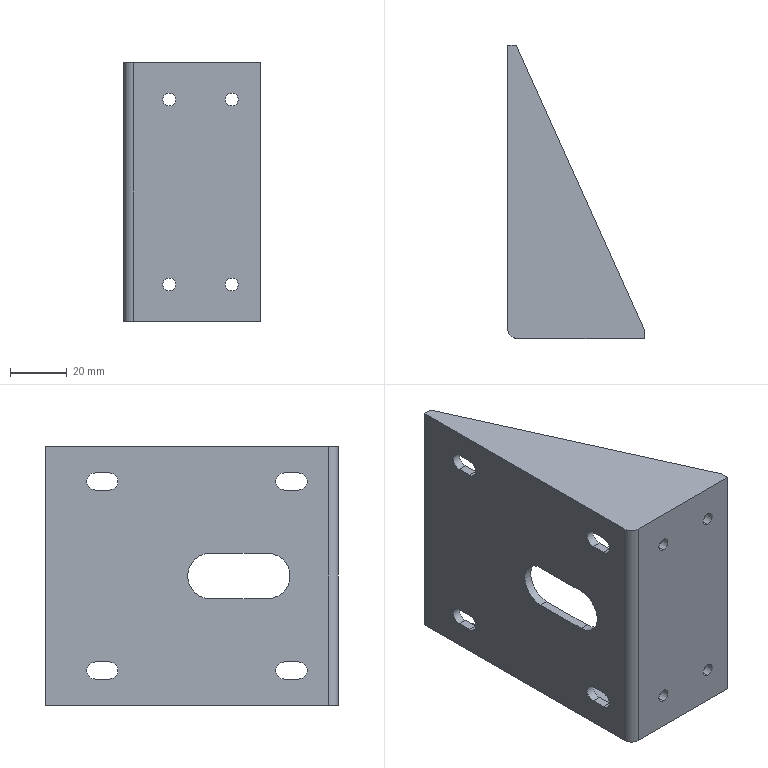Part | SolidWorks | features ICE 4, Cut 1, FlatPattern 1, SMBaseFlange 1, SheetMetal 1 | 1 solid | 42 faces | box 48 x 103 x 91 mm | volume 51216 mm3 | plane 22 | cylinder 20 | commonest cylinder face diameters 4.5 x8 6 x8 16 x2 1 x1 7 x1
STEP:
#1=CARTESIAN_POINT('',(13.,0.,7.75));
#2=VERTEX_POINT('',#1);
#3=CARTESIAN_POINT('',(13.,0.,12.25));
#4=VERTEX_POINT('',#3);
#5=CARTESIAN_POINT('',(13.,0.,10.));
#6=DIRECTION('',(0.,1.,0.));
#7=DIRECTION('',(0.,0.,1.));
#8=AXIS2_PLACEMENT_3D('',#5,#6,#7);
#9=CIRCLE('',#8,2.25);
#10=EDGE_CURVE('',#2,#4,#9,.T.);
#11=ORIENTED_EDGE('',*,*,#10,.T.);
#12=CARTESIAN_POINT('',(13.,-3.,12.25));
#13=VERTEX_POINT('',#12);
#14=CARTESIAN_POINT('',(13.,100.,12.25));
#15=DIRECTION('',(0.,-1.,0.));
#16=VECTOR('',#15,1000.);
#17=LINE('',#14,#16);
#18=EDGE_CURVE('',#4,#13,#17,.T.);
#19=ORIENTED_EDGE('',*,*,#18,.T.);
#20=CARTESIAN_POINT('',(13.,-3.,7.75));
#21=VERTEX_POINT('',#20);
#22=CARTESIAN_POINT('',(13.,-3.,10.));
#23=DIRECTION('',(0.,-1.,0.));
#24=DIRECTION('',(0.,0.,-1.));
#25=AXIS2_PLACEMENT_3D('',#22,#23,#24);
#26=CIRCLE('',#25,2.25);
#27=EDGE_CURVE('',#13,#21,#26,.T.);
#28=ORIENTED_EDGE('',*,*,#27,.T.);
#29=CARTESIAN_POINT('',(13.,100.,7.75));
#30=DIRECTION('',(0.,-1.,0.));
#31=VECTOR('',#30,1000.);
#32=LINE('',#29,#31);
#33=EDGE_CURVE('',#2,#21,#32,.T.);
#34=ORIENTED_EDGE('',*,*,#33,.F.);
#35=EDGE_LOOP('',(#11,#19,#28,#34));
#36=FACE_OUTER_BOUND('',#35,.T.);
#37=CARTESIAN_POINT('',(13.,100.,10.));
#38=DIRECTION('',(0.,-1.,0.));
#39=DIRECTION('',(0.,0.,-1.));
#40=AXIS2_PLACEMENT_3D('',#37,#38,#39);
#41=CYLINDRICAL_SURFACE('',#40,2.25);
#42=ADVANCED_FACE('',(#36),#41,.F.);
#43=CARTESIAN_POINT('',(35.,0.,7.75));
#44=VERTEX_POINT('',#43);
#45=CARTESIAN_POINT('',(35.,0.,12.25));
#46=VERTEX_POINT('',#45);
#47=CARTESIAN_POINT('',(35.,0.,10.));
#48=DIRECTION('',(0.,1.,0.));
#49=DIRECTION('',(0.,0.,1.));
#50=AXIS2_PLACEMENT_3D('',#47,#48,#49);
#51=CIRCLE('',#50,2.25);
#52=EDGE_CURVE('',#44,#46,#51,.T.);
#53=ORIENTED_EDGE('',*,*,#52,.T.);
#54=CARTESIAN_POINT('',(35.,-3.,12.25));
#55=VERTEX_POINT('',#54);
#56=CARTESIAN_POINT('',(35.,100.,12.25));
#57=DIRECTION('',(0.,-1.,0.));
#58=VECTOR('',#57,1000.);
#59=LINE('',#56,#58);
#60=EDGE_CURVE('',#46,#55,#59,.T.);
#61=ORIENTED_EDGE('',*,*,#60,.T.);
#62=CARTESIAN_POINT('',(35.,-3.,7.75));
#63=VERTEX_POINT('',#62);
#64=CARTESIAN_POINT('',(35.,-3.,10.));
#65=DIRECTION('',(0.,-1.,0.));
#66=DIRECTION('',(0.,0.,-1.));
#67=AXIS2_PLACEMENT_3D('',#64,#65,#66);
#68=CIRCLE('',#67,2.25);
#69=EDGE_CURVE('',#55,#63,#68,.T.);
#70=ORIENTED_EDGE('',*,*,#69,.T.);
#71=CARTESIAN_POINT('',(35.,100.,7.75));
#72=DIRECTION('',(0.,-1.,0.));
#73=VECTOR('',#72,1000.);
#74=LINE('',#71,#73);
#75=EDGE_CURVE('',#44,#63,#74,.T.);
#76=ORIENTED_EDGE('',*,*,#75,.F.);
#77=EDGE_LOOP('',(#53,#61,#70,#76));
#78=FACE_OUTER_BOUND('',#77,.T.);
#79=CARTESIAN_POINT('',(35.,100.,10.));
#80=DIRECTION('',(0.,-1.,0.));
#81=DIRECTION('',(0.,0.,-1.));
#82=AXIS2_PLACEMENT_3D('',#79,#80,#81);
#83=CYLINDRICAL_SURFACE('',#82,2.25);
#84=ADVANCED_FACE('',(#78),#83,.F.);
#85=CARTESIAN_POINT('',(35.,0.,72.75));
#86=VERTEX_POINT('',#85);
#87=CARTESIAN_POINT('',(35.,0.,77.25));
#88=VERTEX_POINT('',#87);
#89=CARTESIAN_POINT('',(35.,0.,75.));
#90=DIRECTION('',(0.,1.,0.));
#91=DIRECTION('',(0.,0.,1.));
#92=AXIS2_PLACEMENT_3D('',#89,#90,#91);
#93=CIRCLE('',#92,2.25);
#94=EDGE_CURVE('',#86,#88,#93,.T.);
#95=ORIENTED_EDGE('',*,*,#94,.T.);
#96=CARTESIAN_POINT('',(35.,-3.,77.25));
#97=VERTEX_POINT('',#96);
#98=CARTESIAN_POINT('',(35.,100.,77.25));
#99=DIRECTION('',(0.,-1.,0.));
#100=VECTOR('',#99,1000.);
#101=LINE('',#98,#100);
#102=EDGE_CURVE('',#88,#97,#101,.T.);
#103=ORIENTED_EDGE('',*,*,#102,.T.);
#104=CARTESIAN_POINT('',(35.,-3.,72.75));
#105=VERTEX_POINT('',#104);
#106=CARTESIAN_POINT('',(35.,-3.,75.));
#107=DIRECTION('',(0.,-1.,0.));
#108=DIRECTION('',(0.,0.,-1.));
#109=AXIS2_PLACEMENT_3D('',#106,#107,#108);
#110=CIRCLE('',#109,2.25);
#111=EDGE_CURVE('',#97,#105,#110,.T.);
#112=ORIENTED_EDGE('',*,*,#111,.T.);
#113=CARTESIAN_POINT('',(35.,100.,72.75));
#114=DIRECTION('',(0.,-1.,0.));
#115=VECTOR('',#114,1000.);
#116=LINE('',#113,#115);
#117=EDGE_CURVE('',#86,#105,#116,.T.);
#118=ORIENTED_EDGE('',*,*,#117,.F.);
#119=EDGE_LOOP('',(#95,#103,#112,#118));
#120=FACE_OUTER_BOUND('',#119,.T.);
#121=CARTESIAN_POINT('',(35.,100.,75.));
#122=DIRECTION('',(0.,-1.,0.));
#123=DIRECTION('',(0.,0.,-1.));
#124=AXIS2_PLACEMENT_3D('',#121,#122,#123);
#125=CYLINDRICAL_SURFACE('',#124,2.25);
#126=ADVANCED_FACE('',(#120),#125,.F.);
#127=CARTESIAN_POINT('',(13.,0.,72.75));
#128=VERTEX_POINT('',#127);
#129=CARTESIAN_POINT('',(13.,0.,77.25));
#130=VERTEX_POINT('',#129);
#131=CARTESIAN_POINT('',(13.,0.,75.));
#132=DIRECTION('',(0.,1.,0.));
#133=DIRECTION('',(0.,0.,1.));
#134=AXIS2_PLACEMENT_3D('',#131,#132,#133);
#135=CIRCLE('',#134,2.25);
#136=EDGE_CURVE('',#128,#130,#135,.T.);
#137=ORIENTED_EDGE('',*,*,#136,.T.);
#138=CARTESIAN_POINT('',(13.,-3.,77.25));
#139=VERTEX_POINT('',#138);
#140=CARTESIAN_POINT('',(13.,100.,77.25));
#141=DIRECTION('',(0.,-1.,0.));
#142=VECTOR('',#141,1000.);
#143=LINE('',#140,#142);
#144=EDGE_CURVE('',#130,#139,#143,.T.);
#145=ORIENTED_EDGE('',*,*,#144,.T.);
#146=CARTESIAN_POINT('',(13.,-3.,72.75));
#147=VERTEX_POINT('',#146);
#148=CARTESIAN_POINT('',(13.,-3.,75.));
#149=DIRECTION('',(0.,-1.,0.));
#150=DIRECTION('',(0.,0.,-1.));
#151=AXIS2_PLACEMENT_3D('',#148,#149,#150);
#152=CIRCLE('',#151,2.25);
#153=EDGE_CURVE('',#139,#147,#152,.T.);
#154=ORIENTED_EDGE('',*,*,#153,.T.);
#155=CARTESIAN_POINT('',(13.,100.,72.75));
#156=DIRECTION('',(0.,-1.,0.));
#157=VECTOR('',#156,1000.);
#158=LINE('',#155,#157);
#159=EDGE_CURVE('',#128,#147,#158,.T.);
#160=ORIENTED_EDGE('',*,*,#159,.F.);
#161=EDGE_LOOP('',(#137,#145,#154,#160));
#162=FACE_OUTER_BOUND('',#161,.T.);
#163=CARTESIAN_POINT('',(13.,100.,75.));
#164=DIRECTION('',(0.,-1.,0.));
#165=DIRECTION('',(0.,0.,-1.));
#166=AXIS2_PLACEMENT_3D('',#163,#164,#165);
#167=CYLINDRICAL_SURFACE('',#166,2.25);
#168=ADVANCED_FACE('',(#162),#167,.F.);
#169=CARTESIAN_POINT('',(13.,-3.,10.));
#170=DIRECTION('',(0.,-1.,0.));
#171=DIRECTION('',(0.,0.,-1.));
#172=AXIS2_PLACEMENT_3D('',#169,#170,#171);
#173=CIRCLE('',#172,2.25);
#174=EDGE_CURVE('',#21,#13,#173,.T.);
#175=ORIENTED_EDGE('',*,*,#174,.F.);
#176=ORIENTED_EDGE('',*,*,#27,.F.);
#177=EDGE_LOOP('',(#175,#176));
#178=FACE_BOUND('',#177,.T.);
#179=CARTESIAN_POINT('',(35.,-3.,10.));
#180=DIRECTION('',(0.,-1.,0.));
#181=DIRECTION('',(0.,0.,-1.));
#182=AXIS2_PLACEMENT_3D('',#179,#180,#181);
#183=CIRCLE('',#182,2.25);
#184=EDGE_CURVE('',#63,#55,#183,.T.);
#185=ORIENTED_EDGE('',*,*,#184,.F.);
#186=ORIENTED_EDGE('',*,*,#69,.F.);
#187=EDGE_LOOP('',(#185,#186));
#188=FACE_BOUND('',#187,.T.);
#189=CARTESIAN_POINT('',(35.,-3.,75.));
#190=DIRECTION('',(0.,-1.,0.));
#191=DIRECTION('',(0.,0.,-1.));
#192=AXIS2_PLACEMENT_3D('',#189,#190,#191);
#193=CIRCLE('',#192,2.25);
#194=EDGE_CURVE('',#105,#97,#193,.T.);
#195=ORIENTED_EDGE('',*,*,#194,.F.);
#196=ORIENTED_EDGE('',*,*,#111,.F.);
#197=EDGE_LOOP('',(#195,#196));
#198=FACE_BOUND('',#197,.T.);
#199=CARTESIAN_POINT('',(13.,-3.,75.));
#200=DIRECTION('',(0.,-1.,0.));
#201=DIRECTION('',(0.,0.,-1.));
#202=AXIS2_PLACEMENT_3D('',#199,#200,#201);
#203=CIRCLE('',#202,2.25);
#204=EDGE_CURVE('',#147,#139,#203,.T.);
#205=ORIENTED_EDGE('',*,*,#204,.F.);
#206=ORIENTED_EDGE('',*,*,#153,.F.);
#207=EDGE_LOOP('',(#205,#206));
#208=FACE_BOUND('',#207,.T.);
#209=CARTESIAN_POINT('',(0.5,-3.,88.));
#210=VERTEX_POINT('',#209);
#211=CARTESIAN_POINT('',(0.5,-3.,-3.));
#212=VERTEX_POINT('',#211);
#213=CARTESIAN_POINT('',(0.5,-3.,85.));
#214=DIRECTION('',(0.,0.,-1.));
#215=VECTOR('',#214,1000.);
#216=LINE('',#213,#215);
#217=EDGE_CURVE('',#210,#212,#216,.T.);
#218=ORIENTED_EDGE('',*,*,#217,.T.);
#219=CARTESIAN_POINT('',(45.,-3.,-3.));
#220=VERTEX_POINT('',#219);
#221=CARTESIAN_POINT('',(45.,-3.,-3.));
#222=DIRECTION('',(-1.,0.,0.));
#223=VECTOR('',#222,1000.);
#224=LINE('',#221,#223);
#225=EDGE_CURVE('',#220,#212,#224,.T.);
#226=ORIENTED_EDGE('',*,*,#225,.F.);
#227=CARTESIAN_POINT('',(45.,-3.,88.));
#228=VERTEX_POINT('',#227);
#229=CARTESIAN_POINT('',(45.,-3.,85.));
#230=DIRECTION('',(0.,0.,-1.));
#231=VECTOR('',#230,1000.);
#232=LINE('',#229,#231);
#233=EDGE_CURVE('',#228,#220,#232,.T.);
#234=ORIENTED_EDGE('',*,*,#233,.F.);
#235=CARTESIAN_POINT('',(45.,-3.,88.));
#236=DIRECTION('',(1.,0.,0.));
#237=VECTOR('',#236,1000.);
#238=LINE('',#235,#237);
#239=EDGE_CURVE('',#210,#228,#238,.T.);
#240=ORIENTED_EDGE('',*,*,#239,.F.);
#241=EDGE_LOOP('',(#218,#226,#234,#240));
#242=FACE_OUTER_BOUND('',#241,.T.);
#243=CARTESIAN_POINT('',(0.,-3.,85.));
#244=DIRECTION('',(0.,1.,0.));
#245=DIRECTION('',(0.,0.,1.));
#246=AXIS2_PLACEMENT_3D('',#243,#244,#245);
#247=PLANE('',#246);
#248=ADVANCED_FACE('',(#178,#188,#198,#208,#242),#247,.F.);
#249=ORIENTED_EDGE('',*,*,#233,.T.);
#250=CARTESIAN_POINT('',(45.,0.,-3.));
#251=VERTEX_POINT('',#250);
#252=CARTESIAN_POINT('',(45.,0.,-3.));
#253=DIRECTION('',(0.,-1.,0.));
#254=VECTOR('',#253,1000.);
#255=LINE('',#252,#254);
#256=EDGE_CURVE('',#251,#220,#255,.T.);
#257=ORIENTED_EDGE('',*,*,#256,.F.);
#258=CARTESIAN_POINT('',(45.,0.,0.));
#259=VERTEX_POINT('',#258);
#260=CARTESIAN_POINT('',(45.,0.,-3.));
#261=DIRECTION('',(0.,0.,1.));
#262=VECTOR('',#261,1000.);
#263=LINE('',#260,#262);
#264=EDGE_CURVE('',#251,#259,#263,.T.);
#265=ORIENTED_EDGE('',*,*,#264,.T.);
#266=CARTESIAN_POINT('',(45.,0.,85.));
#267=VERTEX_POINT('',#266);
#268=CARTESIAN_POINT('',(45.,0.,85.));
#269=DIRECTION('',(0.,0.,-1.));
#270=VECTOR('',#269,1000.);
#271=LINE('',#268,#270);
#272=EDGE_CURVE('',#267,#259,#271,.T.);
#273=ORIENTED_EDGE('',*,*,#272,.F.);
#274=CARTESIAN_POINT('',(45.,0.,88.));
#275=VERTEX_POINT('',#274);
#276=CARTESIAN_POINT('',(45.,0.,88.));
#277=DIRECTION('',(0.,0.,-1.));
#278=VECTOR('',#277,1000.);
#279=LINE('',#276,#278);
#280=EDGE_CURVE('',#275,#267,#279,.T.);
#281=ORIENTED_EDGE('',*,*,#280,.F.);
#282=CARTESIAN_POINT('',(45.,0.,88.));
#283=DIRECTION('',(0.,1.,0.));
#284=VECTOR('',#283,1000.);
#285=LINE('',#282,#284);
#286=EDGE_CURVE('',#228,#275,#285,.T.);
#287=ORIENTED_EDGE('',*,*,#286,.F.);
#288=EDGE_LOOP('',(#249,#257,#265,#273,#281,#287));
#289=FACE_OUTER_BOUND('',#288,.T.);
#290=CARTESIAN_POINT('',(45.,0.,85.));
#291=DIRECTION('',(1.,0.,0.));
#292=DIRECTION('',(0.,0.,-1.));
#293=AXIS2_PLACEMENT_3D('',#290,#291,#292);
#294=PLANE('',#293);
#295=ADVANCED_FACE('',(#289),#294,.T.);
#296=ORIENTED_EDGE('',*,*,#10,.F.);
#297=CARTESIAN_POINT('',(13.,0.,10.));
#298=DIRECTION('',(0.,1.,0.));
#299=DIRECTION('',(0.,0.,1.));
#300=AXIS2_PLACEMENT_3D('',#297,#298,#299);
#301=CIRCLE('',#300,2.25);
#302=EDGE_CURVE('',#4,#2,#301,.T.);
#303=ORIENTED_EDGE('',*,*,#302,.F.);
#304=EDGE_LOOP('',(#296,#303));
#305=FACE_BOUND('',#304,.T.);
#306=ORIENTED_EDGE('',*,*,#52,.F.);
#307=CARTESIAN_POINT('',(35.,0.,10.));
#308=DIRECTION('',(0.,1.,0.));
#309=DIRECTION('',(0.,0.,1.));
#310=AXIS2_PLACEMENT_3D('',#307,#308,#309);
#311=CIRCLE('',#310,2.25);
#312=EDGE_CURVE('',#46,#44,#311,.T.);
#313=ORIENTED_EDGE('',*,*,#312,.F.);
#314=EDGE_LOOP('',(#306,#313));
#315=FACE_BOUND('',#314,.T.);
#316=ORIENTED_EDGE('',*,*,#94,.F.);
#317=CARTESIAN_POINT('',(35.,0.,75.));
#318=DIRECTION('',(0.,1.,0.));
#319=DIRECTION('',(0.,0.,1.));
#320=AXIS2_PLACEMENT_3D('',#317,#318,#319);
#321=CIRCLE('',#320,2.25);
#322=EDGE_CURVE('',#88,#86,#321,.T.);
#323=ORIENTED_EDGE('',*,*,#322,.F.);
#324=EDGE_LOOP('',(#316,#323));
#325=FACE_BOUND('',#324,.T.);
#326=ORIENTED_EDGE('',*,*,#136,.F.);
#327=CARTESIAN_POINT('',(13.,0.,75.));
#328=DIRECTION('',(0.,1.,0.));
#329=DIRECTION('',(0.,0.,1.));
#330=AXIS2_PLACEMENT_3D('',#327,#328,#329);
#331=CIRCLE('',#330,2.25);
#332=EDGE_CURVE('',#130,#128,#331,.T.);
#333=ORIENTED_EDGE('',*,*,#332,.F.);
#334=EDGE_LOOP('',(#326,#333));
#335=FACE_BOUND('',#334,.T.);
#336=CARTESIAN_POINT('',(0.5,0.,0.));
#337=VERTEX_POINT('',#336);
#338=CARTESIAN_POINT('',(0.,0.,0.));
#339=DIRECTION('',(1.,0.,0.));
#340=VECTOR('',#339,1000.);
#341=LINE('',#338,#340);
#342=EDGE_CURVE('',#337,#259,#341,.T.);
#343=ORIENTED_EDGE('',*,*,#342,.F.);
#344=CARTESIAN_POINT('',(0.5,0.,85.));
#345=VERTEX_POINT('',#344);
#346=CARTESIAN_POINT('',(0.5,0.,85.));
#347=DIRECTION('',(0.,0.,-1.));
#348=VECTOR('',#347,1000.);
#349=LINE('',#346,#348);
#350=EDGE_CURVE('',#345,#337,#349,.T.);
#351=ORIENTED_EDGE('',*,*,#350,.F.);
#352=CARTESIAN_POINT('',(0.,0.,85.));
#353=DIRECTION('',(1.,0.,0.));
#354=VECTOR('',#353,1000.);
#355=LINE('',#352,#354);
#356=EDGE_CURVE('',#345,#267,#355,.T.);
#357=ORIENTED_EDGE('',*,*,#356,.T.);
#358=ORIENTED_EDGE('',*,*,#272,.T.);
#359=EDGE_LOOP('',(#343,#351,#357,#358));
#360=FACE_OUTER_BOUND('',#359,.T.);
#361=CARTESIAN_POINT('',(0.,0.,85.));
#362=DIRECTION('',(0.,1.,0.));
#363=DIRECTION('',(0.,0.,1.));
#364=AXIS2_PLACEMENT_3D('',#361,#362,#363);
#365=PLANE('',#364);
#366=ADVANCED_FACE('',(#305,#315,#325,#335,#360),#365,.T.);
#367=CARTESIAN_POINT('',(0.,0.5,0.));
#368=VERTEX_POINT('',#367);
#369=CARTESIAN_POINT('',(0.5,0.5,0.));
#370=DIRECTION('',(0.,0.,1.));
#371=DIRECTION('',(-1.,0.,0.));
#372=AXIS2_PLACEMENT_3D('',#369,#370,#371);
#373=CIRCLE('',#372,0.5);
#374=EDGE_CURVE('',#368,#337,#373,.T.);
#375=ORIENTED_EDGE('',*,*,#374,.F.);
#376=CARTESIAN_POINT('',(0.,0.5,85.));
#377=VERTEX_POINT('',#376);
#378=CARTESIAN_POINT('',(0.,0.5,85.));
#379=DIRECTION('',(0.,0.,-1.));
#380=VECTOR('',#379,1000.);
#381=LINE('',#378,#380);
#382=EDGE_CURVE('',#377,#368,#381,.T.);
#383=ORIENTED_EDGE('',*,*,#382,.F.);
#384=CARTESIAN_POINT('',(0.5,0.5,85.));
#385=DIRECTION('',(0.,0.,1.));
#386=DIRECTION('',(-1.,0.,0.));
#387=AXIS2_PLACEMENT_3D('',#384,#385,#386);
#388=CIRCLE('',#387,0.5);
#389=EDGE_CURVE('',#377,#345,#388,.T.);
#390=ORIENTED_EDGE('',*,*,#389,.T.);
#391=ORIENTED_EDGE('',*,*,#350,.T.);
#392=EDGE_LOOP('',(#375,#383,#390,#391));
#393=FACE_OUTER_BOUND('',#392,.T.);
#394=CARTESIAN_POINT('',(0.5,0.5,85.));
#395=DIRECTION('',(0.,0.,-1.));
#396=DIRECTION('',(-1.,0.,0.));
#397=AXIS2_PLACEMENT_3D('',#394,#395,#396);
#398=CYLINDRICAL_SURFACE('',#397,0.5);
#399=ADVANCED_FACE('',(#393),#398,.F.);
#400=CARTESIAN_POINT('',(0.,22.,50.5));
#401=VERTEX_POINT('',#400);
#402=CARTESIAN_POINT('',(0.,22.,34.5));
#403=VERTEX_POINT('',#402);
#404=CARTESIAN_POINT('',(0.,22.,42.5));
#405=DIRECTION('',(1.,0.,0.));
#406=DIRECTION('',(0.,0.,-1.));
#407=AXIS2_PLACEMENT_3D('',#404,#405,#406);
#408=CIRCLE('',#407,8.);
#409=EDGE_CURVE('',#401,#403,#408,.T.);
#410=ORIENTED_EDGE('',*,*,#409,.F.);
#411=CARTESIAN_POINT('',(0.,42.,50.5));
#412=VERTEX_POINT('',#411);
#413=CARTESIAN_POINT('',(0.,0.,50.5));
#414=DIRECTION('',(0.,-1.,0.));
#415=VECTOR('',#414,1000.);
#416=LINE('',#413,#415);
#417=EDGE_CURVE('',#412,#401,#416,.T.);
#418=ORIENTED_EDGE('',*,*,#417,.F.);
#419=CARTESIAN_POINT('',(0.,42.,34.5));
#420=VERTEX_POINT('',#419);
#421=CARTESIAN_POINT('',(0.,42.,42.5));
#422=DIRECTION('',(1.,0.,0.));
#423=DIRECTION('',(0.,0.,-1.));
#424=AXIS2_PLACEMENT_3D('',#421,#422,#423);
#425=CIRCLE('',#424,8.);
#426=EDGE_CURVE('',#420,#412,#425,.T.);
#427=ORIENTED_EDGE('',*,*,#426,.F.);
#428=CARTESIAN_POINT('',(0.,0.,34.5));
#429=DIRECTION('',(0.,1.,0.));
#430=VECTOR('',#429,1000.);
#431=LINE('',#428,#430);
#432=EDGE_CURVE('',#403,#420,#431,.T.);
#433=ORIENTED_EDGE('',*,*,#432,.F.);
#434=EDGE_LOOP('',(#410,#418,#427,#433));
#435=FACE_BOUND('',#434,.T.);
#436=CARTESIAN_POINT('',(0.,16.03,6.265));
#437=VERTEX_POINT('',#436);
#438=CARTESIAN_POINT('',(0.,16.03,12.265));
#439=VERTEX_POINT('',#438);
#440=CARTESIAN_POINT('',(0.,16.03,9.265));
#441=DIRECTION('',(1.,0.,0.));
#442=DIRECTION('',(0.,0.,-1.));
#443=AXIS2_PLACEMENT_3D('',#440,#441,#442);
#444=CIRCLE('',#443,3.);
#445=EDGE_CURVE('',#437,#439,#444,.T.);
#446=ORIENTED_EDGE('',*,*,#445,.F.);
#447=CARTESIAN_POINT('',(0.,11.03,6.265));
#448=VERTEX_POINT('',#447);
#449=CARTESIAN_POINT('',(0.,0.,6.265));
#450=DIRECTION('',(0.,1.,0.));
#451=VECTOR('',#450,1000.);
#452=LINE('',#449,#451);
#453=EDGE_CURVE('',#448,#437,#452,.T.);
#454=ORIENTED_EDGE('',*,*,#453,.F.);
#455=CARTESIAN_POINT('',(0.,11.03,12.265));
#456=VERTEX_POINT('',#455);
#457=CARTESIAN_POINT('',(0.,11.03,9.265));
#458=DIRECTION('',(1.,0.,0.));
#459=DIRECTION('',(0.,0.,-1.));
#460=AXIS2_PLACEMENT_3D('',#457,#458,#459);
#461=CIRCLE('',#460,3.);
#462=EDGE_CURVE('',#456,#448,#461,.T.);
#463=ORIENTED_EDGE('',*,*,#462,.F.);
#464=CARTESIAN_POINT('',(0.,0.,12.265));
#465=DIRECTION('',(0.,-1.,0.));
#466=VECTOR('',#465,1000.);
#467=LINE('',#464,#466);
#468=EDGE_CURVE('',#439,#456,#467,.T.);
#469=ORIENTED_EDGE('',*,*,#468,.F.);
#470=EDGE_LOOP('',(#446,#454,#463,#469));
#471=FACE_BOUND('',#470,.T.);
#472=CARTESIAN_POINT('',(0.,16.03,72.735));
#473=VERTEX_POINT('',#472);
#474=CARTESIAN_POINT('',(0.,16.03,78.735));
#475=VERTEX_POINT('',#474);
#476=CARTESIAN_POINT('',(0.,16.03,75.735));
#477=DIRECTION('',(1.,0.,0.));
#478=DIRECTION('',(0.,0.,-1.));
#479=AXIS2_PLACEMENT_3D('',#476,#477,#478);
#480=CIRCLE('',#479,3.);
#481=EDGE_CURVE('',#473,#475,#480,.T.);
#482=ORIENTED_EDGE('',*,*,#481,.F.);
#483=CARTESIAN_POINT('',(0.,11.03,72.735));
#484=VERTEX_POINT('',#483);
#485=CARTESIAN_POINT('',(0.,0.,72.735));
#486=DIRECTION('',(0.,1.,0.));
#487=VECTOR('',#486,1000.);
#488=LINE('',#485,#487);
#489=EDGE_CURVE('',#484,#473,#488,.T.);
#490=ORIENTED_EDGE('',*,*,#489,.F.);
#491=CARTESIAN_POINT('',(0.,11.03,78.735));
#492=VERTEX_POINT('',#491);
#493=CARTESIAN_POINT('',(0.,11.03,75.735));
#494=DIRECTION('',(1.,0.,0.));
#495=DIRECTION('',(0.,0.,-1.));
#496=AXIS2_PLACEMENT_3D('',#493,#494,#495);
#497=CIRCLE('',#496,3.);
#498=EDGE_CURVE('',#492,#484,#497,.T.);
#499=ORIENTED_EDGE('',*,*,#498,.F.);
#500=CARTESIAN_POINT('',(0.,0.,78.735));
#501=DIRECTION('',(0.,-1.,0.));
#502=VECTOR('',#501,1000.);
#503=LINE('',#500,#502);
#504=EDGE_CURVE('',#475,#492,#503,.T.);
#505=ORIENTED_EDGE('',*,*,#504,.F.);
#506=EDGE_LOOP('',(#482,#490,#499,#505));
#507=FACE_BOUND('',#506,.T.);
#508=CARTESIAN_POINT('',(0.,82.5,72.735));
#509=VERTEX_POINT('',#508);
#510=CARTESIAN_POINT('',(0.,82.5,78.735));
#511=VERTEX_POINT('',#510);
#512=CARTESIAN_POINT('',(0.,82.5,75.735));
#513=DIRECTION('',(1.,0.,0.));
#514=DIRECTION('',(0.,0.,-1.));
#515=AXIS2_PLACEMENT_3D('',#512,#513,#514);
#516=CIRCLE('',#515,3.);
#517=EDGE_CURVE('',#509,#511,#516,.T.);
#518=ORIENTED_EDGE('',*,*,#517,.F.);
#519=CARTESIAN_POINT('',(0.,77.5,72.735));
#520=VERTEX_POINT('',#519);
#521=CARTESIAN_POINT('',(0.,0.,72.735));
#522=DIRECTION('',(0.,1.,0.));
#523=VECTOR('',#522,1000.);
#524=LINE('',#521,#523);
#525=EDGE_CURVE('',#520,#509,#524,.T.);
#526=ORIENTED_EDGE('',*,*,#525,.F.);
#527=CARTESIAN_POINT('',(0.,77.5,78.735));
#528=VERTEX_POINT('',#527);
#529=CARTESIAN_POINT('',(0.,77.5,75.735));
#530=DIRECTION('',(1.,0.,0.));
#531=DIRECTION('',(0.,0.,-1.));
#532=AXIS2_PLACEMENT_3D('',#529,#530,#531);
#533=CIRCLE('',#532,3.);
#534=EDGE_CURVE('',#528,#520,#533,.T.);
#535=ORIENTED_EDGE('',*,*,#534,.F.);
#536=CARTESIAN_POINT('',(0.,0.,78.735));
#537=DIRECTION('',(0.,-1.,0.));
#538=VECTOR('',#537,1000.);
#539=LINE('',#536,#538);
#540=EDGE_CURVE('',#511,#528,#539,.T.);
#541=ORIENTED_EDGE('',*,*,#540,.F.);
#542=EDGE_LOOP('',(#518,#526,#535,#541));
#543=FACE_BOUND('',#542,.T.);
#544=CARTESIAN_POINT('',(0.,82.5,6.265));
#545=VERTEX_POINT('',#544);
#546=CARTESIAN_POINT('',(0.,82.5,12.265));
#547=VERTEX_POINT('',#546);
#548=CARTESIAN_POINT('',(0.,82.5,9.265));
#549=DIRECTION('',(1.,0.,0.));
#550=DIRECTION('',(0.,0.,-1.));
#551=AXIS2_PLACEMENT_3D('',#548,#549,#550);
#552=CIRCLE('',#551,3.);
#553=EDGE_CURVE('',#545,#547,#552,.T.);
#554=ORIENTED_EDGE('',*,*,#553,.F.);
#555=CARTESIAN_POINT('',(0.,77.5,6.265));
#556=VERTEX_POINT('',#555);
#557=CARTESIAN_POINT('',(0.,0.,6.265));
#558=DIRECTION('',(0.,1.,0.));
#559=VECTOR('',#558,1000.);
#560=LINE('',#557,#559);
#561=EDGE_CURVE('',#556,#545,#560,.T.);
#562=ORIENTED_EDGE('',*,*,#561,.F.);
#563=CARTESIAN_POINT('',(0.,77.5,12.265));
#564=VERTEX_POINT('',#563);
#565=CARTESIAN_POINT('',(0.,77.5,9.265));
#566=DIRECTION('',(1.,0.,0.));
#567=DIRECTION('',(0.,0.,-1.));
#568=AXIS2_PLACEMENT_3D('',#565,#566,#567);
#569=CIRCLE('',#568,3.);
#570=EDGE_CURVE('',#564,#556,#569,.T.);
#571=ORIENTED_EDGE('',*,*,#570,.F.);
#572=CARTESIAN_POINT('',(0.,0.,12.265));
#573=DIRECTION('',(0.,-1.,0.));
#574=VECTOR('',#573,1000.);
#575=LINE('',#572,#574);
#576=EDGE_CURVE('',#547,#564,#575,.T.);
#577=ORIENTED_EDGE('',*,*,#576,.F.);
#578=EDGE_LOOP('',(#554,#562,#571,#577));
#579=FACE_BOUND('',#578,.T.);
#580=CARTESIAN_POINT('',(0.,100.,0.));
#581=VERTEX_POINT('',#580);
#582=CARTESIAN_POINT('',(0.,0.,0.));
#583=DIRECTION('',(0.,-1.,0.));
#584=VECTOR('',#583,1000.);
#585=LINE('',#582,#584);
#586=EDGE_CURVE('',#581,#368,#585,.T.);
#587=ORIENTED_EDGE('',*,*,#586,.F.);
#588=CARTESIAN_POINT('',(0.,100.,85.));
#589=VERTEX_POINT('',#588);
#590=CARTESIAN_POINT('',(0.,100.,85.));
#591=DIRECTION('',(0.,0.,-1.));
#592=VECTOR('',#591,1000.);
#593=LINE('',#590,#592);
#594=EDGE_CURVE('',#589,#581,#593,.T.);
#595=ORIENTED_EDGE('',*,*,#594,.F.);
#596=CARTESIAN_POINT('',(0.,0.,85.));
#597=DIRECTION('',(0.,-1.,0.));
#598=VECTOR('',#597,1000.);
#599=LINE('',#596,#598);
#600=EDGE_CURVE('',#589,#377,#599,.T.);
#601=ORIENTED_EDGE('',*,*,#600,.T.);
#602=ORIENTED_EDGE('',*,*,#382,.T.);
#603=EDGE_LOOP('',(#587,#595,#601,#602));
#604=FACE_OUTER_BOUND('',#603,.T.);
#605=CARTESIAN_POINT('',(0.,0.,85.));
#606=DIRECTION('',(1.,0.,0.));
#607=DIRECTION('',(0.,0.,-1.));
#608=AXIS2_PLACEMENT_3D('',#605,#606,#607);
#609=PLANE('',#608);
#610=ADVANCED_FACE('',(#435,#471,#507,#543,#579,#604),#609,.T.);
#611=ORIENTED_EDGE('',*,*,#594,.T.);
#612=CARTESIAN_POINT('',(0.,100.,-3.));
#613=VERTEX_POINT('',#612);
#614=CARTESIAN_POINT('',(0.,100.,-3.));
#615=DIRECTION('',(0.,0.,1.));
#616=VECTOR('',#615,1000.);
#617=LINE('',#614,#616);
#618=EDGE_CURVE('',#613,#581,#617,.T.);
#619=ORIENTED_EDGE('',*,*,#618,.F.);
#620=CARTESIAN_POINT('',(-3.,100.,-3.));
#621=VERTEX_POINT('',#620);
#622=CARTESIAN_POINT('',(-3.,100.,-3.));
#623=DIRECTION('',(1.,0.,0.));
#624=VECTOR('',#623,1000.);
#625=LINE('',#622,#624);
#626=EDGE_CURVE('',#621,#613,#625,.T.);
#627=ORIENTED_EDGE('',*,*,#626,.F.);
#628=CARTESIAN_POINT('',(-3.,100.,88.));
#629=VERTEX_POINT('',#628);
#630=CARTESIAN_POINT('',(-3.,100.,85.));
#631=DIRECTION('',(0.,0.,-1.));
#632=VECTOR('',#631,1000.);
#633=LINE('',#630,#632);
#634=EDGE_CURVE('',#629,#621,#633,.T.);
#635=ORIENTED_EDGE('',*,*,#634,.F.);
#636=CARTESIAN_POINT('',(0.,100.,88.));
#637=VERTEX_POINT('',#636);
#638=CARTESIAN_POINT('',(-3.,100.,88.));
#639=DIRECTION('',(-1.,0.,0.));
#640=VECTOR('',#639,1000.);
#641=LINE('',#638,#640);
#642=EDGE_CURVE('',#637,#629,#641,.T.);
#643=ORIENTED_EDGE('',*,*,#642,.F.);
#644=CARTESIAN_POINT('',(0.,100.,88.));
#645=DIRECTION('',(0.,0.,-1.));
#646=VECTOR('',#645,1000.);
#647=LINE('',#644,#646);
#648=EDGE_CURVE('',#637,#589,#647,.T.);
#649=ORIENTED_EDGE('',*,*,#648,.T.);
#650=EDGE_LOOP('',(#611,#619,#627,#635,#643,#649));
#651=FACE_OUTER_BOUND('',#650,.T.);
#652=CARTESIAN_POINT('',(-3.,100.,85.));
#653=DIRECTION('',(0.,1.,0.));
#654=DIRECTION('',(0.,0.,1.));
#655=AXIS2_PLACEMENT_3D('',#652,#653,#654);
#656=PLANE('',#655);
#657=ADVANCED_FACE('',(#651),#656,.T.);
#658=CARTESIAN_POINT('',(-3.,22.,50.5));
#659=VERTEX_POINT('',#658);
#660=CARTESIAN_POINT('',(-3.,42.,50.5));
#661=VERTEX_POINT('',#660);
#662=CARTESIAN_POINT('',(-3.,22.,50.5));
#663=DIRECTION('',(0.,1.,0.));
#664=VECTOR('',#663,1000.);
#665=LINE('',#662,#664);
#666=EDGE_CURVE('',#659,#661,#665,.T.);
#667=ORIENTED_EDGE('',*,*,#666,.F.);
#668=CARTESIAN_POINT('',(-3.,22.,34.5));
#669=VERTEX_POINT('',#668);
#670=CARTESIAN_POINT('',(-3.,22.,42.5));
#671=DIRECTION('',(-1.,0.,0.));
#672=DIRECTION('',(0.,0.,1.));
#673=AXIS2_PLACEMENT_3D('',#670,#671,#672);
#674=CIRCLE('',#673,8.);
#675=EDGE_CURVE('',#669,#659,#674,.T.);
#676=ORIENTED_EDGE('',*,*,#675,.F.);
#677=CARTESIAN_POINT('',(-3.,42.,34.5));
#678=VERTEX_POINT('',#677);
#679=CARTESIAN_POINT('',(-3.,22.,34.5));
#680=DIRECTION('',(0.,-1.,0.));
#681=VECTOR('',#680,1000.);
#682=LINE('',#679,#681);
#683=EDGE_CURVE('',#678,#669,#682,.T.);
#684=ORIENTED_EDGE('',*,*,#683,.F.);
#685=CARTESIAN_POINT('',(-3.,42.,42.5));
#686=DIRECTION('',(-1.,0.,0.));
#687=DIRECTION('',(0.,0.,1.));
#688=AXIS2_PLACEMENT_3D('',#685,#686,#687);
#689=CIRCLE('',#688,8.);
#690=EDGE_CURVE('',#661,#678,#689,.T.);
#691=ORIENTED_EDGE('',*,*,#690,.F.);
#692=EDGE_LOOP('',(#667,#676,#684,#691));
#693=FACE_BOUND('',#692,.T.);
#694=CARTESIAN_POINT('',(-3.,16.03,6.265));
#695=VERTEX_POINT('',#694);
#696=CARTESIAN_POINT('',(-3.,11.03,6.265));
#697=VERTEX_POINT('',#696);
#698=CARTESIAN_POINT('',(-3.,16.03,6.265));
#699=DIRECTION('',(0.,-1.,0.));
#700=VECTOR('',#699,1000.);
#701=LINE('',#698,#700);
#702=EDGE_CURVE('',#695,#697,#701,.T.);
#703=ORIENTED_EDGE('',*,*,#702,.F.);
#704=CARTESIAN_POINT('',(-3.,16.03,12.265));
#705=VERTEX_POINT('',#704);
#706=CARTESIAN_POINT('',(-3.,16.03,9.265));
#707=DIRECTION('',(-1.,0.,0.));
#708=DIRECTION('',(0.,0.,1.));
#709=AXIS2_PLACEMENT_3D('',#706,#707,#708);
#710=CIRCLE('',#709,3.);
#711=EDGE_CURVE('',#705,#695,#710,.T.);
#712=ORIENTED_EDGE('',*,*,#711,.F.);
#713=CARTESIAN_POINT('',(-3.,11.03,12.265));
#714=VERTEX_POINT('',#713);
#715=CARTESIAN_POINT('',(-3.,16.03,12.265));
#716=DIRECTION('',(0.,1.,0.));
#717=VECTOR('',#716,1000.);
#718=LINE('',#715,#717);
#719=EDGE_CURVE('',#714,#705,#718,.T.);
#720=ORIENTED_EDGE('',*,*,#719,.F.);
#721=CARTESIAN_POINT('',(-3.,11.03,9.265));
#722=DIRECTION('',(-1.,0.,0.));
#723=DIRECTION('',(0.,0.,1.));
#724=AXIS2_PLACEMENT_3D('',#721,#722,#723);
#725=CIRCLE('',#724,3.);
#726=EDGE_CURVE('',#697,#714,#725,.T.);
#727=ORIENTED_EDGE('',*,*,#726,.F.);
#728=EDGE_LOOP('',(#703,#712,#720,#727));
#729=FACE_BOUND('',#728,.T.);
#730=CARTESIAN_POINT('',(-3.,16.03,72.735));
#731=VERTEX_POINT('',#730);
#732=CARTESIAN_POINT('',(-3.,11.03,72.735));
#733=VERTEX_POINT('',#732);
#734=CARTESIAN_POINT('',(-3.,16.03,72.735));
#735=DIRECTION('',(0.,-1.,0.));
#736=VECTOR('',#735,1000.);
#737=LINE('',#734,#736);
#738=EDGE_CURVE('',#731,#733,#737,.T.);
#739=ORIENTED_EDGE('',*,*,#738,.F.);
#740=CARTESIAN_POINT('',(-3.,16.03,78.735));
#741=VERTEX_POINT('',#740);
#742=CARTESIAN_POINT('',(-3.,16.03,75.735));
#743=DIRECTION('',(-1.,0.,0.));
#744=DIRECTION('',(0.,0.,1.));
#745=AXIS2_PLACEMENT_3D('',#742,#743,#744);
#746=CIRCLE('',#745,3.);
#747=EDGE_CURVE('',#741,#731,#746,.T.);
#748=ORIENTED_EDGE('',*,*,#747,.F.);
#749=CARTESIAN_POINT('',(-3.,11.03,78.735));
#750=VERTEX_POINT('',#749);
#751=CARTESIAN_POINT('',(-3.,16.03,78.735));
#752=DIRECTION('',(0.,1.,0.));
#753=VECTOR('',#752,1000.);
#754=LINE('',#751,#753);
#755=EDGE_CURVE('',#750,#741,#754,.T.);
#756=ORIENTED_EDGE('',*,*,#755,.F.);
#757=CARTESIAN_POINT('',(-3.,11.03,75.735));
#758=DIRECTION('',(-1.,0.,0.));
#759=DIRECTION('',(0.,0.,1.));
#760=AXIS2_PLACEMENT_3D('',#757,#758,#759);
#761=CIRCLE('',#760,3.);
#762=EDGE_CURVE('',#733,#750,#761,.T.);
#763=ORIENTED_EDGE('',*,*,#762,.F.);
#764=EDGE_LOOP('',(#739,#748,#756,#763));
#765=FACE_BOUND('',#764,.T.);
#766=CARTESIAN_POINT('',(-3.,82.5,72.735));
#767=VERTEX_POINT('',#766);
#768=CARTESIAN_POINT('',(-3.,77.5,72.735));
#769=VERTEX_POINT('',#768);
#770=CARTESIAN_POINT('',(-3.,82.5,72.735));
#771=DIRECTION('',(0.,-1.,0.));
#772=VECTOR('',#771,1000.);
#773=LINE('',#770,#772);
#774=EDGE_CURVE('',#767,#769,#773,.T.);
#775=ORIENTED_EDGE('',*,*,#774,.F.);
#776=CARTESIAN_POINT('',(-3.,82.5,78.735));
#777=VERTEX_POINT('',#776);
#778=CARTESIAN_POINT('',(-3.,82.5,75.735));
#779=DIRECTION('',(-1.,0.,0.));
#780=DIRECTION('',(0.,0.,1.));
#781=AXIS2_PLACEMENT_3D('',#778,#779,#780);
#782=CIRCLE('',#781,3.);
#783=EDGE_CURVE('',#777,#767,#782,.T.);
#784=ORIENTED_EDGE('',*,*,#783,.F.);
#785=CARTESIAN_POINT('',(-3.,77.5,78.735));
#786=VERTEX_POINT('',#785);
#787=CARTESIAN_POINT('',(-3.,82.5,78.735));
#788=DIRECTION('',(0.,1.,0.));
#789=VECTOR('',#788,1000.);
#790=LINE('',#787,#789);
#791=EDGE_CURVE('',#786,#777,#790,.T.);
#792=ORIENTED_EDGE('',*,*,#791,.F.);
#793=CARTESIAN_POINT('',(-3.,77.5,75.735));
#794=DIRECTION('',(-1.,0.,0.));
#795=DIRECTION('',(0.,0.,1.));
#796=AXIS2_PLACEMENT_3D('',#793,#794,#795);
#797=CIRCLE('',#796,3.);
#798=EDGE_CURVE('',#769,#786,#797,.T.);
#799=ORIENTED_EDGE('',*,*,#798,.F.);
#800=EDGE_LOOP('',(#775,#784,#792,#799));
#801=FACE_BOUND('',#800,.T.);
#802=CARTESIAN_POINT('',(-3.,82.5,6.265));
#803=VERTEX_POINT('',#802);
#804=CARTESIAN_POINT('',(-3.,77.5,6.265));
#805=VERTEX_POINT('',#804);
#806=CARTESIAN_POINT('',(-3.,82.5,6.265));
#807=DIRECTION('',(0.,-1.,0.));
#808=VECTOR('',#807,1000.);
#809=LINE('',#806,#808);
#810=EDGE_CURVE('',#803,#805,#809,.T.);
#811=ORIENTED_EDGE('',*,*,#810,.F.);
#812=CARTESIAN_POINT('',(-3.,82.5,12.265));
#813=VERTEX_POINT('',#812);
#814=CARTESIAN_POINT('',(-3.,82.5,9.265));
#815=DIRECTION('',(-1.,0.,0.));
#816=DIRECTION('',(0.,0.,1.));
#817=AXIS2_PLACEMENT_3D('',#814,#815,#816);
#818=CIRCLE('',#817,3.);
#819=EDGE_CURVE('',#813,#803,#818,.T.);
#820=ORIENTED_EDGE('',*,*,#819,.F.);
#821=CARTESIAN_POINT('',(-3.,77.5,12.265));
#822=VERTEX_POINT('',#821);
#823=CARTESIAN_POINT('',(-3.,82.5,12.265));
#824=DIRECTION('',(0.,1.,0.));
#825=VECTOR('',#824,1000.);
#826=LINE('',#823,#825);
#827=EDGE_CURVE('',#822,#813,#826,.T.);
#828=ORIENTED_EDGE('',*,*,#827,.F.);
#829=CARTESIAN_POINT('',(-3.,77.5,9.265));
#830=DIRECTION('',(-1.,0.,0.));
#831=DIRECTION('',(0.,0.,1.));
#832=AXIS2_PLACEMENT_3D('',#829,#830,#831);
#833=CIRCLE('',#832,3.);
#834=EDGE_CURVE('',#805,#822,#833,.T.);
#835=ORIENTED_EDGE('',*,*,#834,.F.);
#836=EDGE_LOOP('',(#811,#820,#828,#835));
#837=FACE_BOUND('',#836,.T.);
#838=ORIENTED_EDGE('',*,*,#634,.T.);
#839=CARTESIAN_POINT('',(-3.,0.5,-3.));
#840=VERTEX_POINT('',#839);
#841=CARTESIAN_POINT('',(-3.,100.,-3.));
#842=DIRECTION('',(0.,1.,0.));
#843=VECTOR('',#842,1000.);
#844=LINE('',#841,#843);
#845=EDGE_CURVE('',#840,#621,#844,.T.);
#846=ORIENTED_EDGE('',*,*,#845,.F.);
#847=CARTESIAN_POINT('',(-3.,0.5,88.));
#848=VERTEX_POINT('',#847);
#849=CARTESIAN_POINT('',(-3.,0.5,85.));
#850=DIRECTION('',(0.,0.,-1.));
#851=VECTOR('',#850,1000.);
#852=LINE('',#849,#851);
#853=EDGE_CURVE('',#848,#840,#852,.T.);
#854=ORIENTED_EDGE('',*,*,#853,.F.);
#855=CARTESIAN_POINT('',(-3.,0.5,88.));
#856=DIRECTION('',(0.,-1.,0.));
#857=VECTOR('',#856,1000.);
#858=LINE('',#855,#857);
#859=EDGE_CURVE('',#629,#848,#858,.T.);
#860=ORIENTED_EDGE('',*,*,#859,.F.);
#861=EDGE_LOOP('',(#838,#846,#854,#860));
#862=FACE_OUTER_BOUND('',#861,.T.);
#863=CARTESIAN_POINT('',(-3.,0.,85.));
#864=DIRECTION('',(1.,0.,0.));
#865=DIRECTION('',(0.,0.,-1.));
#866=AXIS2_PLACEMENT_3D('',#863,#864,#865);
#867=PLANE('',#866);
#868=ADVANCED_FACE('',(#693,#729,#765,#801,#837,#862),#867,.F.);
#869=ORIENTED_EDGE('',*,*,#853,.T.);
#870=CARTESIAN_POINT('',(0.5,0.5,-3.));
#871=DIRECTION('',(0.,0.,-1.));
#872=DIRECTION('',(1.,0.,0.));
#873=AXIS2_PLACEMENT_3D('',#870,#871,#872);
#874=CIRCLE('',#873,3.5);
#875=EDGE_CURVE('',#212,#840,#874,.T.);
#876=ORIENTED_EDGE('',*,*,#875,.F.);
#877=ORIENTED_EDGE('',*,*,#217,.F.);
#878=CARTESIAN_POINT('',(0.5,0.5,88.));
#879=DIRECTION('',(0.,0.,1.));
#880=DIRECTION('',(1.,0.,0.));
#881=AXIS2_PLACEMENT_3D('',#878,#879,#880);
#882=CIRCLE('',#881,3.5);
#883=EDGE_CURVE('',#848,#210,#882,.T.);
#884=ORIENTED_EDGE('',*,*,#883,.F.);
#885=EDGE_LOOP('',(#869,#876,#877,#884));
#886=FACE_OUTER_BOUND('',#885,.T.);
#887=CARTESIAN_POINT('',(0.5,0.5,85.));
#888=DIRECTION('',(0.,0.,-1.));
#889=DIRECTION('',(-1.,0.,0.));
#890=AXIS2_PLACEMENT_3D('',#887,#888,#889);
#891=CYLINDRICAL_SURFACE('',#890,3.5);
#892=ADVANCED_FACE('',(#886),#891,.T.);
#893=CARTESIAN_POINT('',(0.,100.,85.));
#894=DIRECTION('',(-0.4104,0.9119,0.));
#895=VECTOR('',#894,1000.);
#896=LINE('',#893,#895);
#897=EDGE_CURVE('',#267,#589,#896,.T.);
#898=ORIENTED_EDGE('',*,*,#897,.T.);
#899=ORIENTED_EDGE('',*,*,#648,.F.);
#900=CARTESIAN_POINT('',(0.,100.,88.));
#901=DIRECTION('',(-0.4104,0.9119,0.));
#902=VECTOR('',#901,1000.);
#903=LINE('',#900,#902);
#904=EDGE_CURVE('',#275,#637,#903,.T.);
#905=ORIENTED_EDGE('',*,*,#904,.F.);
#906=ORIENTED_EDGE('',*,*,#280,.T.);
#907=EDGE_LOOP('',(#898,#899,#905,#906));
#908=FACE_OUTER_BOUND('',#907,.T.);
#909=CARTESIAN_POINT('',(0.,100.,88.));
#910=DIRECTION('',(-0.9119,-0.4104,0.));
#911=DIRECTION('',(0.4104,-0.9119,0.));
#912=AXIS2_PLACEMENT_3D('',#909,#910,#911);
#913=PLANE('',#912);
#914=ADVANCED_FACE('',(#908),#913,.F.);
#915=ORIENTED_EDGE('',*,*,#859,.T.);
#916=ORIENTED_EDGE('',*,*,#883,.T.);
#917=ORIENTED_EDGE('',*,*,#239,.T.);
#918=ORIENTED_EDGE('',*,*,#286,.T.);
#919=ORIENTED_EDGE('',*,*,#904,.T.);
#920=ORIENTED_EDGE('',*,*,#642,.T.);
#921=EDGE_LOOP('',(#915,#916,#917,#918,#919,#920));
#922=FACE_OUTER_BOUND('',#921,.T.);
#923=CARTESIAN_POINT('',(0.5,0.5,88.));
#924=DIRECTION('',(0.,0.,1.));
#925=DIRECTION('',(1.,0.,0.));
#926=AXIS2_PLACEMENT_3D('',#923,#924,#925);
#927=PLANE('',#926);
#928=ADVANCED_FACE('',(#922),#927,.T.);
#929=ORIENTED_EDGE('',*,*,#356,.F.);
#930=ORIENTED_EDGE('',*,*,#389,.F.);
#931=ORIENTED_EDGE('',*,*,#600,.F.);
#932=ORIENTED_EDGE('',*,*,#897,.F.);
#933=EDGE_LOOP('',(#929,#930,#931,#932));
#934=FACE_OUTER_BOUND('',#933,.T.);
#935=CARTESIAN_POINT('',(0.5,0.5,85.));
#936=DIRECTION('',(0.,0.,1.));
#937=DIRECTION('',(1.,0.,0.));
#938=AXIS2_PLACEMENT_3D('',#935,#936,#937);
#939=PLANE('',#938);
#940=ADVANCED_FACE('',(#934),#939,.F.);
#941=CARTESIAN_POINT('',(0.,100.,0.));
#942=DIRECTION('',(0.4104,-0.9119,0.));
#943=VECTOR('',#942,1000.);
#944=LINE('',#941,#943);
#945=EDGE_CURVE('',#581,#259,#944,.T.);
#946=ORIENTED_EDGE('',*,*,#945,.T.);
#947=ORIENTED_EDGE('',*,*,#264,.F.);
#948=CARTESIAN_POINT('',(0.,100.,-3.));
#949=DIRECTION('',(0.4104,-0.9119,0.));
#950=VECTOR('',#949,1000.);
#951=LINE('',#948,#950);
#952=EDGE_CURVE('',#613,#251,#951,.T.);
#953=ORIENTED_EDGE('',*,*,#952,.F.);
#954=ORIENTED_EDGE('',*,*,#618,.T.);
#955=EDGE_LOOP('',(#946,#947,#953,#954));
#956=FACE_OUTER_BOUND('',#955,.T.);
#957=CARTESIAN_POINT('',(0.,100.,-3.));
#958=DIRECTION('',(-0.9119,-0.4104,0.));
#959=DIRECTION('',(0.4104,-0.9119,0.));
#960=AXIS2_PLACEMENT_3D('',#957,#958,#959);
#961=PLANE('',#960);
#962=ADVANCED_FACE('',(#956),#961,.F.);
#963=ORIENTED_EDGE('',*,*,#845,.T.);
#964=ORIENTED_EDGE('',*,*,#626,.T.);
#965=ORIENTED_EDGE('',*,*,#952,.T.);
#966=ORIENTED_EDGE('',*,*,#256,.T.);
#967=ORIENTED_EDGE('',*,*,#225,.T.);
#968=ORIENTED_EDGE('',*,*,#875,.T.);
#969=EDGE_LOOP('',(#963,#964,#965,#966,#967,#968));
#970=FACE_OUTER_BOUND('',#969,.T.);
#971=CARTESIAN_POINT('',(0.5,0.5,-3.));
#972=DIRECTION('',(0.,0.,1.));
#973=DIRECTION('',(1.,0.,0.));
#974=AXIS2_PLACEMENT_3D('',#971,#972,#973);
#975=PLANE('',#974);
#976=ADVANCED_FACE('',(#970),#975,.F.);
#977=ORIENTED_EDGE('',*,*,#374,.T.);
#978=ORIENTED_EDGE('',*,*,#342,.T.);
#979=ORIENTED_EDGE('',*,*,#945,.F.);
#980=ORIENTED_EDGE('',*,*,#586,.T.);
#981=EDGE_LOOP('',(#977,#978,#979,#980));
#982=FACE_OUTER_BOUND('',#981,.T.);
#983=CARTESIAN_POINT('',(0.5,0.5,0.));
#984=DIRECTION('',(0.,0.,1.));
#985=DIRECTION('',(1.,0.,0.));
#986=AXIS2_PLACEMENT_3D('',#983,#984,#985);
#987=PLANE('',#986);
#988=ADVANCED_FACE('',(#982),#987,.T.);
#989=ORIENTED_EDGE('',*,*,#553,.T.);
#990=CARTESIAN_POINT('',(7.,82.5,12.265));
#991=DIRECTION('',(-1.,0.,0.));
#992=VECTOR('',#991,1000.);
#993=LINE('',#990,#992);
#994=EDGE_CURVE('',#547,#813,#993,.T.);
#995=ORIENTED_EDGE('',*,*,#994,.T.);
#996=ORIENTED_EDGE('',*,*,#819,.T.);
#997=CARTESIAN_POINT('',(7.,82.5,6.265));
#998=DIRECTION('',(-1.,0.,0.));
#999=VECTOR('',#998,1000.);
#1000=LINE('',#997,#999);
#1001=EDGE_CURVE('',#545,#803,#1000,.T.);
#1002=ORIENTED_EDGE('',*,*,#1001,.F.);
#1003=EDGE_LOOP('',(#989,#995,#996,#1002));
#1004=FACE_OUTER_BOUND('',#1003,.T.);
#1005=CARTESIAN_POINT('',(7.,82.5,9.265));
#1006=DIRECTION('',(-1.,0.,0.));
#1007=DIRECTION('',(0.,0.,1.));
#1008=AXIS2_PLACEMENT_3D('',#1005,#1006,#1007);
#1009=CYLINDRICAL_SURFACE('',#1008,3.);
#1010=ADVANCED_FACE('',(#1004),#1009,.F.);
#1011=ORIENTED_EDGE('',*,*,#576,.T.);
#1012=CARTESIAN_POINT('',(7.,77.5,12.265));
#1013=DIRECTION('',(-1.,0.,0.));
#1014=VECTOR('',#1013,1000.);
#1015=LINE('',#1012,#1014);
#1016=EDGE_CURVE('',#564,#822,#1015,.T.);
#1017=ORIENTED_EDGE('',*,*,#1016,.T.);
#1018=ORIENTED_EDGE('',*,*,#827,.T.);
#1019=ORIENTED_EDGE('',*,*,#994,.F.);
#1020=EDGE_LOOP('',(#1011,#1017,#1018,#1019));
#1021=FACE_OUTER_BOUND('',#1020,.T.);
#1022=CARTESIAN_POINT('',(7.,82.5,12.265));
#1023=DIRECTION('',(0.,0.,1.));
#1024=DIRECTION('',(0.,-1.,0.));
#1025=AXIS2_PLACEMENT_3D('',#1022,#1023,#1024);
#1026=PLANE('',#1025);
#1027=ADVANCED_FACE('',(#1021),#1026,.F.);
#1028=ORIENTED_EDGE('',*,*,#570,.T.);
#1029=CARTESIAN_POINT('',(7.,77.5,6.265));
#1030=DIRECTION('',(-1.,0.,0.));
#1031=VECTOR('',#1030,1000.);
#1032=LINE('',#1029,#1031);
#1033=EDGE_CURVE('',#556,#805,#1032,.T.);
#1034=ORIENTED_EDGE('',*,*,#1033,.T.);
#1035=ORIENTED_EDGE('',*,*,#834,.T.);
#1036=ORIENTED_EDGE('',*,*,#1016,.F.);
#1037=EDGE_LOOP('',(#1028,#1034,#1035,#1036));
#1038=FACE_OUTER_BOUND('',#1037,.T.);
#1039=CARTESIAN_POINT('',(7.,77.5,9.265));
#1040=DIRECTION('',(-1.,0.,0.));
#1041=DIRECTION('',(0.,0.,1.));
#1042=AXIS2_PLACEMENT_3D('',#1039,#1040,#1041);
#1043=CYLINDRICAL_SURFACE('',#1042,3.);
#1044=ADVANCED_FACE('',(#1038),#1043,.F.);
#1045=ORIENTED_EDGE('',*,*,#561,.T.);
#1046=ORIENTED_EDGE('',*,*,#1001,.T.);
#1047=ORIENTED_EDGE('',*,*,#810,.T.);
#1048=ORIENTED_EDGE('',*,*,#1033,.F.);
#1049=EDGE_LOOP('',(#1045,#1046,#1047,#1048));
#1050=FACE_OUTER_BOUND('',#1049,.T.);
#1051=CARTESIAN_POINT('',(7.,82.5,6.265));
#1052=DIRECTION('',(0.,0.,-1.));
#1053=DIRECTION('',(0.,1.,0.));
#1054=AXIS2_PLACEMENT_3D('',#1051,#1052,#1053);
#1055=PLANE('',#1054);
#1056=ADVANCED_FACE('',(#1050),#1055,.F.);
#1057=ORIENTED_EDGE('',*,*,#517,.T.);
#1058=CARTESIAN_POINT('',(7.,82.5,78.735));
#1059=DIRECTION('',(-1.,0.,0.));
#1060=VECTOR('',#1059,1000.);
#1061=LINE('',#1058,#1060);
#1062=EDGE_CURVE('',#511,#777,#1061,.T.);
#1063=ORIENTED_EDGE('',*,*,#1062,.T.);
#1064=ORIENTED_EDGE('',*,*,#783,.T.);
#1065=CARTESIAN_POINT('',(7.,82.5,72.735));
#1066=DIRECTION('',(-1.,0.,0.));
#1067=VECTOR('',#1066,1000.);
#1068=LINE('',#1065,#1067);
#1069=EDGE_CURVE('',#509,#767,#1068,.T.);
#1070=ORIENTED_EDGE('',*,*,#1069,.F.);
#1071=EDGE_LOOP('',(#1057,#1063,#1064,#1070));
#1072=FACE_OUTER_BOUND('',#1071,.T.);
#1073=CARTESIAN_POINT('',(7.,82.5,75.735));
#1074=DIRECTION('',(-1.,0.,0.));
#1075=DIRECTION('',(0.,0.,1.));
#1076=AXIS2_PLACEMENT_3D('',#1073,#1074,#1075);
#1077=CYLINDRICAL_SURFACE('',#1076,3.);
#1078=ADVANCED_FACE('',(#1072),#1077,.F.);
#1079=ORIENTED_EDGE('',*,*,#540,.T.);
#1080=CARTESIAN_POINT('',(7.,77.5,78.735));
#1081=DIRECTION('',(-1.,0.,0.));
#1082=VECTOR('',#1081,1000.);
#1083=LINE('',#1080,#1082);
#1084=EDGE_CURVE('',#528,#786,#1083,.T.);
#1085=ORIENTED_EDGE('',*,*,#1084,.T.);
#1086=ORIENTED_EDGE('',*,*,#791,.T.);
#1087=ORIENTED_EDGE('',*,*,#1062,.F.);
#1088=EDGE_LOOP('',(#1079,#1085,#1086,#1087));
#1089=FACE_OUTER_BOUND('',#1088,.T.);
#1090=CARTESIAN_POINT('',(7.,82.5,78.735));
#1091=DIRECTION('',(0.,0.,1.));
#1092=DIRECTION('',(1.,0.,0.));
#1093=AXIS2_PLACEMENT_3D('',#1090,#1091,#1092);
#1094=PLANE('',#1093);
#1095=ADVANCED_FACE('',(#1089),#1094,.F.);
#1096=ORIENTED_EDGE('',*,*,#534,.T.);
#1097=CARTESIAN_POINT('',(7.,77.5,72.735));
#1098=DIRECTION('',(-1.,0.,0.));
#1099=VECTOR('',#1098,1000.);
#1100=LINE('',#1097,#1099);
#1101=EDGE_CURVE('',#520,#769,#1100,.T.);
#1102=ORIENTED_EDGE('',*,*,#1101,.T.);
#1103=ORIENTED_EDGE('',*,*,#798,.T.);
#1104=ORIENTED_EDGE('',*,*,#1084,.F.);
#1105=EDGE_LOOP('',(#1096,#1102,#1103,#1104));
#1106=FACE_OUTER_BOUND('',#1105,.T.);
#1107=CARTESIAN_POINT('',(7.,77.5,75.735));
#1108=DIRECTION('',(-1.,0.,0.));
#1109=DIRECTION('',(0.,0.,1.));
#1110=AXIS2_PLACEMENT_3D('',#1107,#1108,#1109);
#1111=CYLINDRICAL_SURFACE('',#1110,3.);
#1112=ADVANCED_FACE('',(#1106),#1111,.F.);
#1113=ORIENTED_EDGE('',*,*,#525,.T.);
#1114=ORIENTED_EDGE('',*,*,#1069,.T.);
#1115=ORIENTED_EDGE('',*,*,#774,.T.);
#1116=ORIENTED_EDGE('',*,*,#1101,.F.);
#1117=EDGE_LOOP('',(#1113,#1114,#1115,#1116));
#1118=FACE_OUTER_BOUND('',#1117,.T.);
#1119=CARTESIAN_POINT('',(7.,82.5,72.735));
#1120=DIRECTION('',(0.,0.,-1.));
#1121=DIRECTION('',(-1.,0.,0.));
#1122=AXIS2_PLACEMENT_3D('',#1119,#1120,#1121);
#1123=PLANE('',#1122);
#1124=ADVANCED_FACE('',(#1118),#1123,.F.);
#1125=ORIENTED_EDGE('',*,*,#481,.T.);
#1126=CARTESIAN_POINT('',(7.,16.03,78.735));
#1127=DIRECTION('',(-1.,0.,0.));
#1128=VECTOR('',#1127,1000.);
#1129=LINE('',#1126,#1128);
#1130=EDGE_CURVE('',#475,#741,#1129,.T.);
#1131=ORIENTED_EDGE('',*,*,#1130,.T.);
#1132=ORIENTED_EDGE('',*,*,#747,.T.);
#1133=CARTESIAN_POINT('',(7.,16.03,72.735));
#1134=DIRECTION('',(-1.,0.,0.));
#1135=VECTOR('',#1134,1000.);
#1136=LINE('',#1133,#1135);
#1137=EDGE_CURVE('',#473,#731,#1136,.T.);
#1138=ORIENTED_EDGE('',*,*,#1137,.F.);
#1139=EDGE_LOOP('',(#1125,#1131,#1132,#1138));
#1140=FACE_OUTER_BOUND('',#1139,.T.);
#1141=CARTESIAN_POINT('',(7.,16.03,75.735));
#1142=DIRECTION('',(-1.,0.,0.));
#1143=DIRECTION('',(0.,0.,1.));
#1144=AXIS2_PLACEMENT_3D('',#1141,#1142,#1143);
#1145=CYLINDRICAL_SURFACE('',#1144,3.);
#1146=ADVANCED_FACE('',(#1140),#1145,.F.);
#1147=ORIENTED_EDGE('',*,*,#504,.T.);
#1148=CARTESIAN_POINT('',(7.,11.03,78.735));
#1149=DIRECTION('',(-1.,0.,0.));
#1150=VECTOR('',#1149,1000.);
#1151=LINE('',#1148,#1150);
#1152=EDGE_CURVE('',#492,#750,#1151,.T.);
#1153=ORIENTED_EDGE('',*,*,#1152,.T.);
#1154=ORIENTED_EDGE('',*,*,#755,.T.);
#1155=ORIENTED_EDGE('',*,*,#1130,.F.);
#1156=EDGE_LOOP('',(#1147,#1153,#1154,#1155));
#1157=FACE_OUTER_BOUND('',#1156,.T.);
#1158=CARTESIAN_POINT('',(7.,16.03,78.735));
#1159=DIRECTION('',(0.,0.,1.));
#1160=DIRECTION('',(1.,0.,0.));
#1161=AXIS2_PLACEMENT_3D('',#1158,#1159,#1160);
#1162=PLANE('',#1161);
#1163=ADVANCED_FACE('',(#1157),#1162,.F.);
#1164=ORIENTED_EDGE('',*,*,#498,.T.);
#1165=CARTESIAN_POINT('',(7.,11.03,72.735));
#1166=DIRECTION('',(-1.,0.,0.));
#1167=VECTOR('',#1166,1000.);
#1168=LINE('',#1165,#1167);
#1169=EDGE_CURVE('',#484,#733,#1168,.T.);
#1170=ORIENTED_EDGE('',*,*,#1169,.T.);
#1171=ORIENTED_EDGE('',*,*,#762,.T.);
#1172=ORIENTED_EDGE('',*,*,#1152,.F.);
#1173=EDGE_LOOP('',(#1164,#1170,#1171,#1172));
#1174=FACE_OUTER_BOUND('',#1173,.T.);
#1175=CARTESIAN_POINT('',(7.,11.03,75.735));
#1176=DIRECTION('',(-1.,0.,0.));
#1177=DIRECTION('',(0.,0.,1.));
#1178=AXIS2_PLACEMENT_3D('',#1175,#1176,#1177);
#1179=CYLINDRICAL_SURFACE('',#1178,3.);
#1180=ADVANCED_FACE('',(#1174),#1179,.F.);
#1181=ORIENTED_EDGE('',*,*,#489,.T.);
#1182=ORIENTED_EDGE('',*,*,#1137,.T.);
#1183=ORIENTED_EDGE('',*,*,#738,.T.);
#1184=ORIENTED_EDGE('',*,*,#1169,.F.);
#1185=EDGE_LOOP('',(#1181,#1182,#1183,#1184));
#1186=FACE_OUTER_BOUND('',#1185,.T.);
#1187=CARTESIAN_POINT('',(7.,16.03,72.735));
#1188=DIRECTION('',(0.,0.,-1.));
#1189=DIRECTION('',(-1.,0.,0.));
#1190=AXIS2_PLACEMENT_3D('',#1187,#1188,#1189);
#1191=PLANE('',#1190);
#1192=ADVANCED_FACE('',(#1186),#1191,.F.);
#1193=ORIENTED_EDGE('',*,*,#445,.T.);
#1194=CARTESIAN_POINT('',(7.,16.03,12.265));
#1195=DIRECTION('',(-1.,0.,0.));
#1196=VECTOR('',#1195,1000.);
#1197=LINE('',#1194,#1196);
#1198=EDGE_CURVE('',#439,#705,#1197,.T.);
#1199=ORIENTED_EDGE('',*,*,#1198,.T.);
#1200=ORIENTED_EDGE('',*,*,#711,.T.);
#1201=CARTESIAN_POINT('',(7.,16.03,6.265));
#1202=DIRECTION('',(-1.,0.,0.));
#1203=VECTOR('',#1202,1000.);
#1204=LINE('',#1201,#1203);
#1205=EDGE_CURVE('',#437,#695,#1204,.T.);
#1206=ORIENTED_EDGE('',*,*,#1205,.F.);
#1207=EDGE_LOOP('',(#1193,#1199,#1200,#1206));
#1208=FACE_OUTER_BOUND('',#1207,.T.);
#1209=CARTESIAN_POINT('',(7.,16.03,9.265));
#1210=DIRECTION('',(-1.,0.,0.));
#1211=DIRECTION('',(0.,0.,1.));
#1212=AXIS2_PLACEMENT_3D('',#1209,#1210,#1211);
#1213=CYLINDRICAL_SURFACE('',#1212,3.);
#1214=ADVANCED_FACE('',(#1208),#1213,.F.);
#1215=ORIENTED_EDGE('',*,*,#468,.T.);
#1216=CARTESIAN_POINT('',(7.,11.03,12.265));
#1217=DIRECTION('',(-1.,0.,0.));
#1218=VECTOR('',#1217,1000.);
#1219=LINE('',#1216,#1218);
#1220=EDGE_CURVE('',#456,#714,#1219,.T.);
#1221=ORIENTED_EDGE('',*,*,#1220,.T.);
#1222=ORIENTED_EDGE('',*,*,#719,.T.);
#1223=ORIENTED_EDGE('',*,*,#1198,.F.);
#1224=EDGE_LOOP('',(#1215,#1221,#1222,#1223));
#1225=FACE_OUTER_BOUND('',#1224,.T.);
#1226=CARTESIAN_POINT('',(7.,16.03,12.265));
#1227=DIRECTION('',(0.,0.,1.));
#1228=DIRECTION('',(0.,-1.,0.));
#1229=AXIS2_PLACEMENT_3D('',#1226,#1227,#1228);
#1230=PLANE('',#1229);
#1231=ADVANCED_FACE('',(#1225),#1230,.F.);
#1232=ORIENTED_EDGE('',*,*,#462,.T.);
#1233=CARTESIAN_POINT('',(7.,11.03,6.265));
#1234=DIRECTION('',(-1.,0.,0.));
#1235=VECTOR('',#1234,1000.);
#1236=LINE('',#1233,#1235);
#1237=EDGE_CURVE('',#448,#697,#1236,.T.);
#1238=ORIENTED_EDGE('',*,*,#1237,.T.);
#1239=ORIENTED_EDGE('',*,*,#726,.T.);
#1240=ORIENTED_EDGE('',*,*,#1220,.F.);
#1241=EDGE_LOOP('',(#1232,#1238,#1239,#1240));
#1242=FACE_OUTER_BOUND('',#1241,.T.);
#1243=CARTESIAN_POINT('',(7.,11.03,9.265));
#1244=DIRECTION('',(-1.,0.,0.));
#1245=DIRECTION('',(0.,0.,1.));
#1246=AXIS2_PLACEMENT_3D('',#1243,#1244,#1245);
#1247=CYLINDRICAL_SURFACE('',#1246,3.);
#1248=ADVANCED_FACE('',(#1242),#1247,.F.);
#1249=ORIENTED_EDGE('',*,*,#453,.T.);
#1250=ORIENTED_EDGE('',*,*,#1205,.T.);
#1251=ORIENTED_EDGE('',*,*,#702,.T.);
#1252=ORIENTED_EDGE('',*,*,#1237,.F.);
#1253=EDGE_LOOP('',(#1249,#1250,#1251,#1252));
#1254=FACE_OUTER_BOUND('',#1253,.T.);
#1255=CARTESIAN_POINT('',(7.,16.03,6.265));
#1256=DIRECTION('',(0.,0.,-1.));
#1257=DIRECTION('',(0.,1.,0.));
#1258=AXIS2_PLACEMENT_3D('',#1255,#1256,#1257);
#1259=PLANE('',#1258);
#1260=ADVANCED_FACE('',(#1254),#1259,.F.);
#1261=ORIENTED_EDGE('',*,*,#144,.F.);
#1262=ORIENTED_EDGE('',*,*,#332,.T.);
#1263=ORIENTED_EDGE('',*,*,#159,.T.);
#1264=ORIENTED_EDGE('',*,*,#204,.T.);
#1265=EDGE_LOOP('',(#1261,#1262,#1263,#1264));
#1266=FACE_OUTER_BOUND('',#1265,.T.);
#1267=CARTESIAN_POINT('',(13.,100.,75.));
#1268=DIRECTION('',(0.,-1.,0.));
#1269=DIRECTION('',(0.,0.,-1.));
#1270=AXIS2_PLACEMENT_3D('',#1267,#1268,#1269);
#1271=CYLINDRICAL_SURFACE('',#1270,2.25);
#1272=ADVANCED_FACE('',(#1266),#1271,.F.);
#1273=ORIENTED_EDGE('',*,*,#102,.F.);
#1274=ORIENTED_EDGE('',*,*,#322,.T.);
#1275=ORIENTED_EDGE('',*,*,#117,.T.);
#1276=ORIENTED_EDGE('',*,*,#194,.T.);
#1277=EDGE_LOOP('',(#1273,#1274,#1275,#1276));
#1278=FACE_OUTER_BOUND('',#1277,.T.);
#1279=CARTESIAN_POINT('',(35.,100.,75.));
#1280=DIRECTION('',(0.,-1.,0.));
#1281=DIRECTION('',(0.,0.,-1.));
#1282=AXIS2_PLACEMENT_3D('',#1279,#1280,#1281);
#1283=CYLINDRICAL_SURFACE('',#1282,2.25);
#1284=ADVANCED_FACE('',(#1278),#1283,.F.);
#1285=ORIENTED_EDGE('',*,*,#60,.F.);
#1286=ORIENTED_EDGE('',*,*,#312,.T.);
#1287=ORIENTED_EDGE('',*,*,#75,.T.);
#1288=ORIENTED_EDGE('',*,*,#184,.T.);
#1289=EDGE_LOOP('',(#1285,#1286,#1287,#1288));
#1290=FACE_OUTER_BOUND('',#1289,.T.);
#1291=CARTESIAN_POINT('',(35.,100.,10.));
#1292=DIRECTION('',(0.,-1.,0.));
#1293=DIRECTION('',(0.,0.,-1.));
#1294=AXIS2_PLACEMENT_3D('',#1291,#1292,#1293);
#1295=CYLINDRICAL_SURFACE('',#1294,2.25);
#1296=ADVANCED_FACE('',(#1290),#1295,.F.);
#1297=ORIENTED_EDGE('',*,*,#18,.F.);
#1298=ORIENTED_EDGE('',*,*,#302,.T.);
#1299=ORIENTED_EDGE('',*,*,#33,.T.);
#1300=ORIENTED_EDGE('',*,*,#174,.T.);
#1301=EDGE_LOOP('',(#1297,#1298,#1299,#1300));
#1302=FACE_OUTER_BOUND('',#1301,.T.);
#1303=CARTESIAN_POINT('',(13.,100.,10.));
#1304=DIRECTION('',(0.,-1.,0.));
#1305=DIRECTION('',(0.,0.,-1.));
#1306=AXIS2_PLACEMENT_3D('',#1303,#1304,#1305);
#1307=CYLINDRICAL_SURFACE('',#1306,2.25);
#1308=ADVANCED_FACE('',(#1302),#1307,.F.);
#1309=ORIENTED_EDGE('',*,*,#409,.T.);
#1310=CARTESIAN_POINT('',(7.,22.,34.5));
#1311=DIRECTION('',(-1.,0.,0.));
#1312=VECTOR('',#1311,1000.);
#1313=LINE('',#1310,#1312);
#1314=EDGE_CURVE('',#403,#669,#1313,.T.);
#1315=ORIENTED_EDGE('',*,*,#1314,.T.);
#1316=ORIENTED_EDGE('',*,*,#675,.T.);
#1317=CARTESIAN_POINT('',(7.,22.,50.5));
#1318=DIRECTION('',(-1.,0.,0.));
#1319=VECTOR('',#1318,1000.);
#1320=LINE('',#1317,#1319);
#1321=EDGE_CURVE('',#401,#659,#1320,.T.);
#1322=ORIENTED_EDGE('',*,*,#1321,.F.);
#1323=EDGE_LOOP('',(#1309,#1315,#1316,#1322));
#1324=FACE_OUTER_BOUND('',#1323,.T.);
#1325=CARTESIAN_POINT('',(7.,22.,42.5));
#1326=DIRECTION('',(-1.,0.,0.));
#1327=DIRECTION('',(0.,0.,1.));
#1328=AXIS2_PLACEMENT_3D('',#1325,#1326,#1327);
#1329=CYLINDRICAL_SURFACE('',#1328,8.);
#1330=ADVANCED_FACE('',(#1324),#1329,.F.);
#1331=ORIENTED_EDGE('',*,*,#432,.T.);
#1332=CARTESIAN_POINT('',(7.,42.,34.5));
#1333=DIRECTION('',(-1.,0.,0.));
#1334=VECTOR('',#1333,1000.);
#1335=LINE('',#1332,#1334);
#1336=EDGE_CURVE('',#420,#678,#1335,.T.);
#1337=ORIENTED_EDGE('',*,*,#1336,.T.);
#1338=ORIENTED_EDGE('',*,*,#683,.T.);
#1339=ORIENTED_EDGE('',*,*,#1314,.F.);
#1340=EDGE_LOOP('',(#1331,#1337,#1338,#1339));
#1341=FACE_OUTER_BOUND('',#1340,.T.);
#1342=CARTESIAN_POINT('',(7.,22.,34.5));
#1343=DIRECTION('',(0.,0.,-1.));
#1344=DIRECTION('',(-1.,0.,0.));
#1345=AXIS2_PLACEMENT_3D('',#1342,#1343,#1344);
#1346=PLANE('',#1345);
#1347=ADVANCED_FACE('',(#1341),#1346,.F.);
#1348=ORIENTED_EDGE('',*,*,#426,.T.);
#1349=CARTESIAN_POINT('',(7.,42.,50.5));
#1350=DIRECTION('',(-1.,0.,0.));
#1351=VECTOR('',#1350,1000.);
#1352=LINE('',#1349,#1351);
#1353=EDGE_CURVE('',#412,#661,#1352,.T.);
#1354=ORIENTED_EDGE('',*,*,#1353,.T.);
#1355=ORIENTED_EDGE('',*,*,#690,.T.);
#1356=ORIENTED_EDGE('',*,*,#1336,.F.);
#1357=EDGE_LOOP('',(#1348,#1354,#1355,#1356));
#1358=FACE_OUTER_BOUND('',#1357,.T.);
#1359=CARTESIAN_POINT('',(7.,42.,42.5));
#1360=DIRECTION('',(-1.,0.,0.));
#1361=DIRECTION('',(0.,0.,1.));
#1362=AXIS2_PLACEMENT_3D('',#1359,#1360,#1361);
#1363=CYLINDRICAL_SURFACE('',#1362,8.);
#1364=ADVANCED_FACE('',(#1358),#1363,.F.);
#1365=ORIENTED_EDGE('',*,*,#417,.T.);
#1366=ORIENTED_EDGE('',*,*,#1321,.T.);
#1367=ORIENTED_EDGE('',*,*,#666,.T.);
#1368=ORIENTED_EDGE('',*,*,#1353,.F.);
#1369=EDGE_LOOP('',(#1365,#1366,#1367,#1368));
#1370=FACE_OUTER_BOUND('',#1369,.T.);
#1371=CARTESIAN_POINT('',(7.,22.,50.5));
#1372=DIRECTION('',(0.,0.,1.));
#1373=DIRECTION('',(1.,0.,0.));
#1374=AXIS2_PLACEMENT_3D('',#1371,#1372,#1373);
#1375=PLANE('',#1374);
#1376=ADVANCED_FACE('',(#1370),#1375,.F.);
#1377=CLOSED_SHELL('',(#42,#84,#126,#168,#248,#295,#366,#399,#610,#657,#868,#892,#914,#928,#940,#962,#976,#988,#1010,#1027,#1044,#1056,#1078,#1095,#1112,#1124,#1146,#1163,#1180,#1192,#1214,#1231,#1248,#1260,#1272,#1284,#1296,#1308,#1330,#1347,#1364,#1376));
#1378=MANIFOLD_SOLID_BREP('',#1377);
#1379=CARTESIAN_POINT('',(0.,0.,0.));
#1380=DIRECTION('',(0.,0.,1.));
#1381=DIRECTION('',(1.,0.,0.));
#1382=AXIS2_PLACEMENT_3D('',#1379,#1380,#1381);
#1383=(LENGTH_UNIT()NAMED_UNIT(*)SI_UNIT(.MILLI.,.METRE.));
#1384=UNCERTAINTY_MEASURE_WITH_UNIT(LENGTH_MEASURE(0.00001),#1383,'','');
#1385=(NAMED_UNIT(*)PLANE_ANGLE_UNIT()SI_UNIT($,.RADIAN.));
#1386=(NAMED_UNIT(*)SI_UNIT($,.STERADIAN.)SOLID_ANGLE_UNIT());
#1387=(GEOMETRIC_REPRESENTATION_CONTEXT(3)GLOBAL_UNCERTAINTY_ASSIGNED_CONTEXT((#1384))GLOBAL_UNIT_ASSIGNED_CONTEXT((#1383,#1385,#1386))REPRESENTATION_CONTEXT('',''));
#1388=ADVANCED_BREP_SHAPE_REPRESENTATION('',(#1378,#1382),#1387);